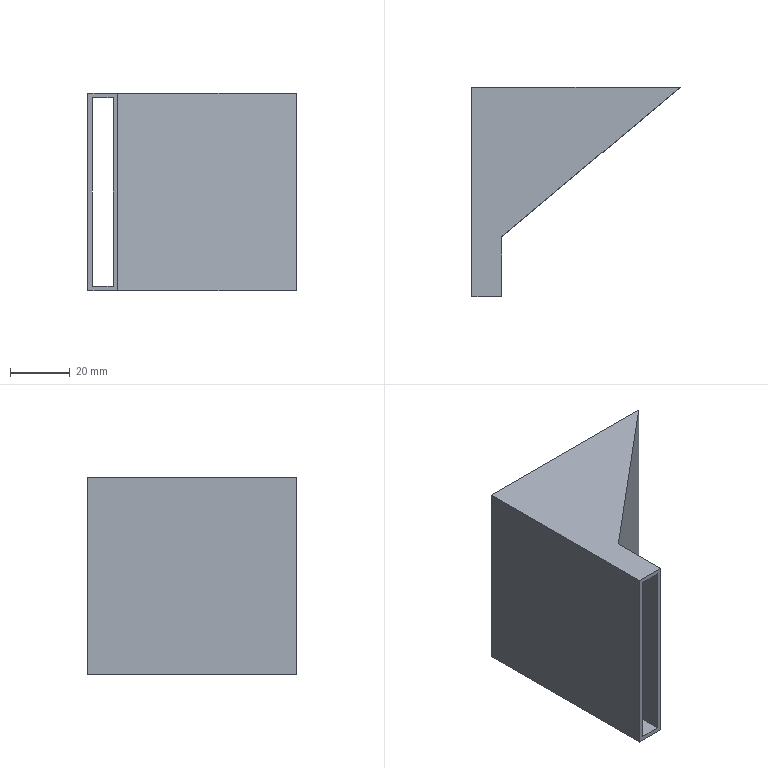Part | STEP file | Hopper | 1 solid | 12 faces | box 69.588 x 70 x 66 mm | volume 22407 mm3 | plane 12
STEP:
#1=CARTESIAN_POINT('',(0.,0.,-33.));
#2=VERTEX_POINT('',#1);
#3=CARTESIAN_POINT('',(10.,0.,-33.));
#4=VERTEX_POINT('',#3);
#5=CARTESIAN_POINT('',(10.,0.,-33.));
#6=DIRECTION('',(1.,0.,0.));
#7=VECTOR('',#6,1000.);
#8=LINE('',#5,#7);
#9=EDGE_CURVE('',#2,#4,#8,.T.);
#10=ORIENTED_EDGE('',*,*,#9,.T.);
#11=CARTESIAN_POINT('',(10.,0.,33.));
#12=VERTEX_POINT('',#11);
#13=CARTESIAN_POINT('',(10.,0.,33.));
#14=DIRECTION('',(0.,0.,-1.));
#15=VECTOR('',#14,1000.);
#16=LINE('',#13,#15);
#17=EDGE_CURVE('',#12,#4,#16,.T.);
#18=ORIENTED_EDGE('',*,*,#17,.F.);
#19=CARTESIAN_POINT('',(0.,0.,33.));
#20=VERTEX_POINT('',#19);
#21=CARTESIAN_POINT('',(10.,0.,33.));
#22=DIRECTION('',(1.,0.,0.));
#23=VECTOR('',#22,1000.);
#24=LINE('',#21,#23);
#25=EDGE_CURVE('',#20,#12,#24,.T.);
#26=ORIENTED_EDGE('',*,*,#25,.F.);
#27=CARTESIAN_POINT('',(0.,0.,33.));
#28=DIRECTION('',(0.,0.,-1.));
#29=VECTOR('',#28,1000.);
#30=LINE('',#27,#29);
#31=EDGE_CURVE('',#20,#2,#30,.T.);
#32=ORIENTED_EDGE('',*,*,#31,.T.);
#33=EDGE_LOOP('',(#10,#18,#26,#32));
#34=FACE_OUTER_BOUND('',#33,.T.);
#35=CARTESIAN_POINT('',(1.5,0.,-31.5));
#36=VERTEX_POINT('',#35);
#37=CARTESIAN_POINT('',(8.5,0.,-31.5));
#38=VERTEX_POINT('',#37);
#39=CARTESIAN_POINT('',(0.,0.,-31.5));
#40=DIRECTION('',(1.,0.,0.));
#41=VECTOR('',#40,1000.);
#42=LINE('',#39,#41);
#43=EDGE_CURVE('',#36,#38,#42,.T.);
#44=ORIENTED_EDGE('',*,*,#43,.F.);
#45=CARTESIAN_POINT('',(1.5,0.,31.5));
#46=VERTEX_POINT('',#45);
#47=CARTESIAN_POINT('',(1.5,0.,33.));
#48=DIRECTION('',(0.,0.,-1.));
#49=VECTOR('',#48,1000.);
#50=LINE('',#47,#49);
#51=EDGE_CURVE('',#46,#36,#50,.T.);
#52=ORIENTED_EDGE('',*,*,#51,.F.);
#53=CARTESIAN_POINT('',(8.5,0.,31.5));
#54=VERTEX_POINT('',#53);
#55=CARTESIAN_POINT('',(0.,0.,31.5));
#56=DIRECTION('',(1.,0.,0.));
#57=VECTOR('',#56,1000.);
#58=LINE('',#55,#57);
#59=EDGE_CURVE('',#46,#54,#58,.T.);
#60=ORIENTED_EDGE('',*,*,#59,.T.);
#61=CARTESIAN_POINT('',(8.5,0.,33.));
#62=DIRECTION('',(0.,0.,-1.));
#63=VECTOR('',#62,1000.);
#64=LINE('',#61,#63);
#65=EDGE_CURVE('',#54,#38,#64,.T.);
#66=ORIENTED_EDGE('',*,*,#65,.T.);
#67=EDGE_LOOP('',(#44,#52,#60,#66));
#68=FACE_BOUND('',#67,.T.);
#69=CARTESIAN_POINT('',(10.,0.,33.));
#70=DIRECTION('',(0.,1.,0.));
#71=DIRECTION('',(0.,0.,1.));
#72=AXIS2_PLACEMENT_3D('',#69,#70,#71);
#73=PLANE('',#72);
#74=ADVANCED_FACE('',(#34,#68),#73,.F.);
#75=CARTESIAN_POINT('',(69.588,70.,-33.));
#76=VERTEX_POINT('',#75);
#77=CARTESIAN_POINT('',(0.,70.,-33.));
#78=VERTEX_POINT('',#77);
#79=CARTESIAN_POINT('',(0.,70.,-33.));
#80=DIRECTION('',(-1.,0.,0.));
#81=VECTOR('',#80,1000.);
#82=LINE('',#79,#81);
#83=EDGE_CURVE('',#76,#78,#82,.T.);
#84=ORIENTED_EDGE('',*,*,#83,.T.);
#85=CARTESIAN_POINT('',(0.,70.,33.));
#86=VERTEX_POINT('',#85);
#87=CARTESIAN_POINT('',(0.,70.,33.));
#88=DIRECTION('',(0.,0.,-1.));
#89=VECTOR('',#88,1000.);
#90=LINE('',#87,#89);
#91=EDGE_CURVE('',#86,#78,#90,.T.);
#92=ORIENTED_EDGE('',*,*,#91,.F.);
#93=CARTESIAN_POINT('',(69.588,70.,33.));
#94=VERTEX_POINT('',#93);
#95=CARTESIAN_POINT('',(0.,70.,33.));
#96=DIRECTION('',(-1.,0.,0.));
#97=VECTOR('',#96,1000.);
#98=LINE('',#95,#97);
#99=EDGE_CURVE('',#94,#86,#98,.T.);
#100=ORIENTED_EDGE('',*,*,#99,.F.);
#101=CARTESIAN_POINT('',(69.588,70.,33.));
#102=DIRECTION('',(0.,0.,-1.));
#103=VECTOR('',#102,1000.);
#104=LINE('',#101,#103);
#105=EDGE_CURVE('',#94,#76,#104,.T.);
#106=ORIENTED_EDGE('',*,*,#105,.T.);
#107=EDGE_LOOP('',(#84,#92,#100,#106));
#108=FACE_OUTER_BOUND('',#107,.T.);
#109=CARTESIAN_POINT('',(67.254,70.,-31.5));
#110=VERTEX_POINT('',#109);
#111=CARTESIAN_POINT('',(1.5,70.,-31.5));
#112=VERTEX_POINT('',#111);
#113=CARTESIAN_POINT('',(0.,70.,-31.5));
#114=DIRECTION('',(-1.,0.,0.));
#115=VECTOR('',#114,1000.);
#116=LINE('',#113,#115);
#117=EDGE_CURVE('',#110,#112,#116,.T.);
#118=ORIENTED_EDGE('',*,*,#117,.F.);
#119=CARTESIAN_POINT('',(67.254,70.,31.5));
#120=VERTEX_POINT('',#119);
#121=CARTESIAN_POINT('',(67.254,70.,33.));
#122=DIRECTION('',(0.,0.,-1.));
#123=VECTOR('',#122,1000.);
#124=LINE('',#121,#123);
#125=EDGE_CURVE('',#120,#110,#124,.T.);
#126=ORIENTED_EDGE('',*,*,#125,.F.);
#127=CARTESIAN_POINT('',(1.5,70.,31.5));
#128=VERTEX_POINT('',#127);
#129=CARTESIAN_POINT('',(0.,70.,31.5));
#130=DIRECTION('',(-1.,0.,0.));
#131=VECTOR('',#130,1000.);
#132=LINE('',#129,#131);
#133=EDGE_CURVE('',#120,#128,#132,.T.);
#134=ORIENTED_EDGE('',*,*,#133,.T.);
#135=CARTESIAN_POINT('',(1.5,70.,33.));
#136=DIRECTION('',(0.,0.,-1.));
#137=VECTOR('',#136,1000.);
#138=LINE('',#135,#137);
#139=EDGE_CURVE('',#128,#112,#138,.T.);
#140=ORIENTED_EDGE('',*,*,#139,.T.);
#141=EDGE_LOOP('',(#118,#126,#134,#140));
#142=FACE_BOUND('',#141,.T.);
#143=CARTESIAN_POINT('',(0.,70.,33.));
#144=DIRECTION('',(0.,-1.,0.));
#145=DIRECTION('',(0.,0.,-1.));
#146=AXIS2_PLACEMENT_3D('',#143,#144,#145);
#147=PLANE('',#146);
#148=ADVANCED_FACE('',(#108,#142),#147,.F.);
#149=CARTESIAN_POINT('',(10.,20.,-33.));
#150=VERTEX_POINT('',#149);
#151=CARTESIAN_POINT('',(10.,20.,-33.));
#152=DIRECTION('',(0.,1.,0.));
#153=VECTOR('',#152,1000.);
#154=LINE('',#151,#153);
#155=EDGE_CURVE('',#4,#150,#154,.T.);
#156=ORIENTED_EDGE('',*,*,#155,.T.);
#157=CARTESIAN_POINT('',(10.,20.,33.));
#158=VERTEX_POINT('',#157);
#159=CARTESIAN_POINT('',(10.,20.,33.));
#160=DIRECTION('',(0.,0.,-1.));
#161=VECTOR('',#160,1000.);
#162=LINE('',#159,#161);
#163=EDGE_CURVE('',#158,#150,#162,.T.);
#164=ORIENTED_EDGE('',*,*,#163,.F.);
#165=CARTESIAN_POINT('',(10.,20.,33.));
#166=DIRECTION('',(0.,1.,0.));
#167=VECTOR('',#166,1000.);
#168=LINE('',#165,#167);
#169=EDGE_CURVE('',#12,#158,#168,.T.);
#170=ORIENTED_EDGE('',*,*,#169,.F.);
#171=ORIENTED_EDGE('',*,*,#17,.T.);
#172=EDGE_LOOP('',(#156,#164,#170,#171));
#173=FACE_OUTER_BOUND('',#172,.T.);
#174=CARTESIAN_POINT('',(10.,20.,33.));
#175=DIRECTION('',(-1.,0.,0.));
#176=DIRECTION('',(0.,-1.,0.));
#177=AXIS2_PLACEMENT_3D('',#174,#175,#176);
#178=PLANE('',#177);
#179=ADVANCED_FACE('',(#173),#178,.F.);
#180=CARTESIAN_POINT('',(69.588,70.,-33.));
#181=DIRECTION('',(0.766,0.6428,0.));
#182=VECTOR('',#181,1000.);
#183=LINE('',#180,#182);
#184=EDGE_CURVE('',#150,#76,#183,.T.);
#185=ORIENTED_EDGE('',*,*,#184,.T.);
#186=ORIENTED_EDGE('',*,*,#105,.F.);
#187=CARTESIAN_POINT('',(69.588,70.,33.));
#188=DIRECTION('',(0.766,0.6428,0.));
#189=VECTOR('',#188,1000.);
#190=LINE('',#187,#189);
#191=EDGE_CURVE('',#158,#94,#190,.T.);
#192=ORIENTED_EDGE('',*,*,#191,.F.);
#193=ORIENTED_EDGE('',*,*,#163,.T.);
#194=EDGE_LOOP('',(#185,#186,#192,#193));
#195=FACE_OUTER_BOUND('',#194,.T.);
#196=CARTESIAN_POINT('',(69.588,70.,33.));
#197=DIRECTION('',(-0.6428,0.766,0.));
#198=DIRECTION('',(-0.766,-0.6428,0.));
#199=AXIS2_PLACEMENT_3D('',#196,#197,#198);
#200=PLANE('',#199);
#201=ADVANCED_FACE('',(#195),#200,.F.);
#202=CARTESIAN_POINT('',(0.,0.,-33.));
#203=DIRECTION('',(0.,-1.,0.));
#204=VECTOR('',#203,1000.);
#205=LINE('',#202,#204);
#206=EDGE_CURVE('',#78,#2,#205,.T.);
#207=ORIENTED_EDGE('',*,*,#206,.T.);
#208=ORIENTED_EDGE('',*,*,#31,.F.);
#209=CARTESIAN_POINT('',(0.,0.,33.));
#210=DIRECTION('',(0.,-1.,0.));
#211=VECTOR('',#210,1000.);
#212=LINE('',#209,#211);
#213=EDGE_CURVE('',#86,#20,#212,.T.);
#214=ORIENTED_EDGE('',*,*,#213,.F.);
#215=ORIENTED_EDGE('',*,*,#91,.T.);
#216=EDGE_LOOP('',(#207,#208,#214,#215));
#217=FACE_OUTER_BOUND('',#216,.T.);
#218=CARTESIAN_POINT('',(0.,0.,33.));
#219=DIRECTION('',(1.,0.,0.));
#220=DIRECTION('',(0.,0.,-1.));
#221=AXIS2_PLACEMENT_3D('',#218,#219,#220);
#222=PLANE('',#221);
#223=ADVANCED_FACE('',(#217),#222,.F.);
#224=ORIENTED_EDGE('',*,*,#25,.T.);
#225=ORIENTED_EDGE('',*,*,#169,.T.);
#226=ORIENTED_EDGE('',*,*,#191,.T.);
#227=ORIENTED_EDGE('',*,*,#99,.T.);
#228=ORIENTED_EDGE('',*,*,#213,.T.);
#229=EDGE_LOOP('',(#224,#225,#226,#227,#228));
#230=FACE_OUTER_BOUND('',#229,.T.);
#231=CARTESIAN_POINT('',(0.,0.,33.));
#232=DIRECTION('',(0.,0.,-1.));
#233=DIRECTION('',(-1.,0.,0.));
#234=AXIS2_PLACEMENT_3D('',#231,#232,#233);
#235=PLANE('',#234);
#236=ADVANCED_FACE('',(#230),#235,.F.);
#237=ORIENTED_EDGE('',*,*,#9,.F.);
#238=ORIENTED_EDGE('',*,*,#206,.F.);
#239=ORIENTED_EDGE('',*,*,#83,.F.);
#240=ORIENTED_EDGE('',*,*,#184,.F.);
#241=ORIENTED_EDGE('',*,*,#155,.F.);
#242=EDGE_LOOP('',(#237,#238,#239,#240,#241));
#243=FACE_OUTER_BOUND('',#242,.T.);
#244=CARTESIAN_POINT('',(0.,0.,-33.));
#245=DIRECTION('',(0.,0.,-1.));
#246=DIRECTION('',(-1.,0.,0.));
#247=AXIS2_PLACEMENT_3D('',#244,#245,#246);
#248=PLANE('',#247);
#249=ADVANCED_FACE('',(#243),#248,.T.);
#250=CARTESIAN_POINT('',(8.5,20.699,-31.5));
#251=VERTEX_POINT('',#250);
#252=CARTESIAN_POINT('',(8.5,0.,-31.5));
#253=DIRECTION('',(0.,1.,0.));
#254=VECTOR('',#253,1000.);
#255=LINE('',#252,#254);
#256=EDGE_CURVE('',#38,#251,#255,.T.);
#257=ORIENTED_EDGE('',*,*,#256,.F.);
#258=ORIENTED_EDGE('',*,*,#65,.F.);
#259=CARTESIAN_POINT('',(8.5,20.699,31.5));
#260=VERTEX_POINT('',#259);
#261=CARTESIAN_POINT('',(8.5,0.,31.5));
#262=DIRECTION('',(0.,1.,0.));
#263=VECTOR('',#262,1000.);
#264=LINE('',#261,#263);
#265=EDGE_CURVE('',#54,#260,#264,.T.);
#266=ORIENTED_EDGE('',*,*,#265,.T.);
#267=CARTESIAN_POINT('',(8.5,20.699,33.));
#268=DIRECTION('',(0.,0.,-1.));
#269=VECTOR('',#268,1000.);
#270=LINE('',#267,#269);
#271=EDGE_CURVE('',#260,#251,#270,.T.);
#272=ORIENTED_EDGE('',*,*,#271,.T.);
#273=EDGE_LOOP('',(#257,#258,#266,#272));
#274=FACE_OUTER_BOUND('',#273,.T.);
#275=CARTESIAN_POINT('',(8.5,20.,33.));
#276=DIRECTION('',(-1.,0.,0.));
#277=DIRECTION('',(0.,-1.,0.));
#278=AXIS2_PLACEMENT_3D('',#275,#276,#277);
#279=PLANE('',#278);
#280=ADVANCED_FACE('',(#274),#279,.T.);
#281=CARTESIAN_POINT('',(-6.68,7.962,-31.5));
#282=DIRECTION('',(0.766,0.6428,0.));
#283=VECTOR('',#282,1000.);
#284=LINE('',#281,#283);
#285=EDGE_CURVE('',#251,#110,#284,.T.);
#286=ORIENTED_EDGE('',*,*,#285,.F.);
#287=ORIENTED_EDGE('',*,*,#271,.F.);
#288=CARTESIAN_POINT('',(-6.68,7.962,31.5));
#289=DIRECTION('',(0.766,0.6428,0.));
#290=VECTOR('',#289,1000.);
#291=LINE('',#288,#290);
#292=EDGE_CURVE('',#260,#120,#291,.T.);
#293=ORIENTED_EDGE('',*,*,#292,.T.);
#294=ORIENTED_EDGE('',*,*,#125,.T.);
#295=EDGE_LOOP('',(#286,#287,#293,#294));
#296=FACE_OUTER_BOUND('',#295,.T.);
#297=CARTESIAN_POINT('',(68.623,71.149,33.));
#298=DIRECTION('',(-0.6428,0.766,0.));
#299=DIRECTION('',(-0.766,-0.6428,0.));
#300=AXIS2_PLACEMENT_3D('',#297,#298,#299);
#301=PLANE('',#300);
#302=ADVANCED_FACE('',(#296),#301,.T.);
#303=CARTESIAN_POINT('',(1.5,0.,-31.5));
#304=DIRECTION('',(0.,-1.,0.));
#305=VECTOR('',#304,1000.);
#306=LINE('',#303,#305);
#307=EDGE_CURVE('',#112,#36,#306,.T.);
#308=ORIENTED_EDGE('',*,*,#307,.F.);
#309=ORIENTED_EDGE('',*,*,#139,.F.);
#310=CARTESIAN_POINT('',(1.5,0.,31.5));
#311=DIRECTION('',(0.,-1.,0.));
#312=VECTOR('',#311,1000.);
#313=LINE('',#310,#312);
#314=EDGE_CURVE('',#128,#46,#313,.T.);
#315=ORIENTED_EDGE('',*,*,#314,.T.);
#316=ORIENTED_EDGE('',*,*,#51,.T.);
#317=EDGE_LOOP('',(#308,#309,#315,#316));
#318=FACE_OUTER_BOUND('',#317,.T.);
#319=CARTESIAN_POINT('',(1.5,0.,33.));
#320=DIRECTION('',(1.,0.,0.));
#321=DIRECTION('',(0.,0.,-1.));
#322=AXIS2_PLACEMENT_3D('',#319,#320,#321);
#323=PLANE('',#322);
#324=ADVANCED_FACE('',(#318),#323,.T.);
#325=ORIENTED_EDGE('',*,*,#59,.F.);
#326=ORIENTED_EDGE('',*,*,#314,.F.);
#327=ORIENTED_EDGE('',*,*,#133,.F.);
#328=ORIENTED_EDGE('',*,*,#292,.F.);
#329=ORIENTED_EDGE('',*,*,#265,.F.);
#330=EDGE_LOOP('',(#325,#326,#327,#328,#329));
#331=FACE_OUTER_BOUND('',#330,.T.);
#332=CARTESIAN_POINT('',(0.,0.,31.5));
#333=DIRECTION('',(0.,0.,-1.));
#334=DIRECTION('',(-1.,0.,0.));
#335=AXIS2_PLACEMENT_3D('',#332,#333,#334);
#336=PLANE('',#335);
#337=ADVANCED_FACE('',(#331),#336,.T.);
#338=ORIENTED_EDGE('',*,*,#43,.T.);
#339=ORIENTED_EDGE('',*,*,#256,.T.);
#340=ORIENTED_EDGE('',*,*,#285,.T.);
#341=ORIENTED_EDGE('',*,*,#117,.T.);
#342=ORIENTED_EDGE('',*,*,#307,.T.);
#343=EDGE_LOOP('',(#338,#339,#340,#341,#342));
#344=FACE_OUTER_BOUND('',#343,.T.);
#345=CARTESIAN_POINT('',(0.,0.,-31.5));
#346=DIRECTION('',(0.,0.,-1.));
#347=DIRECTION('',(-1.,0.,0.));
#348=AXIS2_PLACEMENT_3D('',#345,#346,#347);
#349=PLANE('',#348);
#350=ADVANCED_FACE('',(#344),#349,.F.);
#351=CLOSED_SHELL('',(#74,#148,#179,#201,#223,#236,#249,#280,#302,#324,#337,#350));
#352=MANIFOLD_SOLID_BREP('',#351);
#353=CARTESIAN_POINT('',(0.,0.,0.));
#354=DIRECTION('',(0.,0.,1.));
#355=DIRECTION('',(1.,0.,0.));
#356=AXIS2_PLACEMENT_3D('',#353,#354,#355);
#357=(LENGTH_UNIT()NAMED_UNIT(*)SI_UNIT(.MILLI.,.METRE.));
#358=UNCERTAINTY_MEASURE_WITH_UNIT(LENGTH_MEASURE(0.00001),#357,'','');
#359=(NAMED_UNIT(*)PLANE_ANGLE_UNIT()SI_UNIT($,.RADIAN.));
#360=(NAMED_UNIT(*)SI_UNIT($,.STERADIAN.)SOLID_ANGLE_UNIT());
#361=(GEOMETRIC_REPRESENTATION_CONTEXT(3)GLOBAL_UNCERTAINTY_ASSIGNED_CONTEXT((#358))GLOBAL_UNIT_ASSIGNED_CONTEXT((#357,#359,#360))REPRESENTATION_CONTEXT('',''));
#362=ADVANCED_BREP_SHAPE_REPRESENTATION('',(#352,#356),#361);